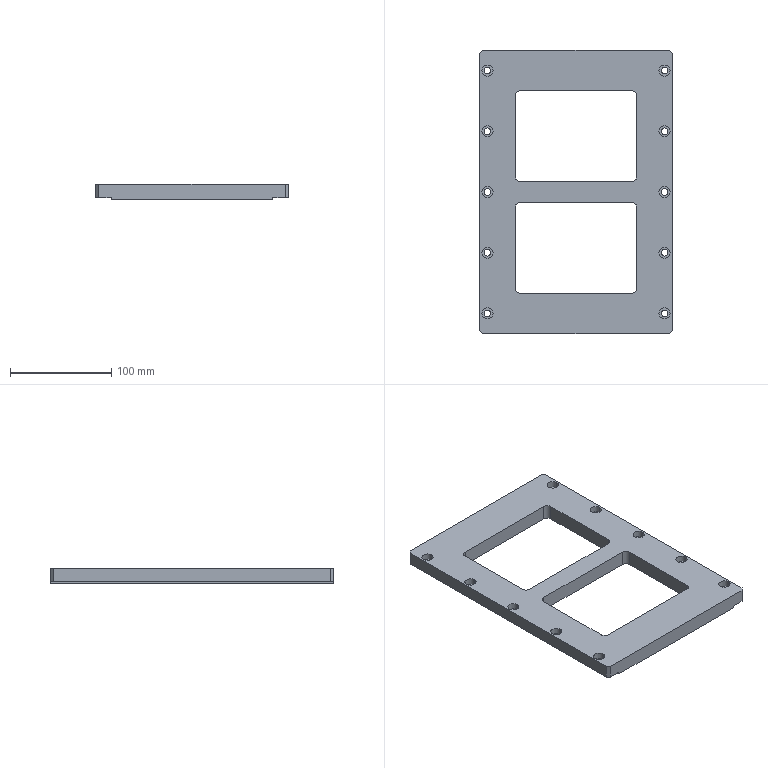Part | STEP file | 10-11 lift fixing plate | 1 solid | 96 faces | box 190 x 280 x 15 mm | volume 448559 mm3 | cylinder 56 | plane 32 | cone 8 | commonest cylinder face diameters 6.6 x20 11 x20 4.2 x8 10 x8